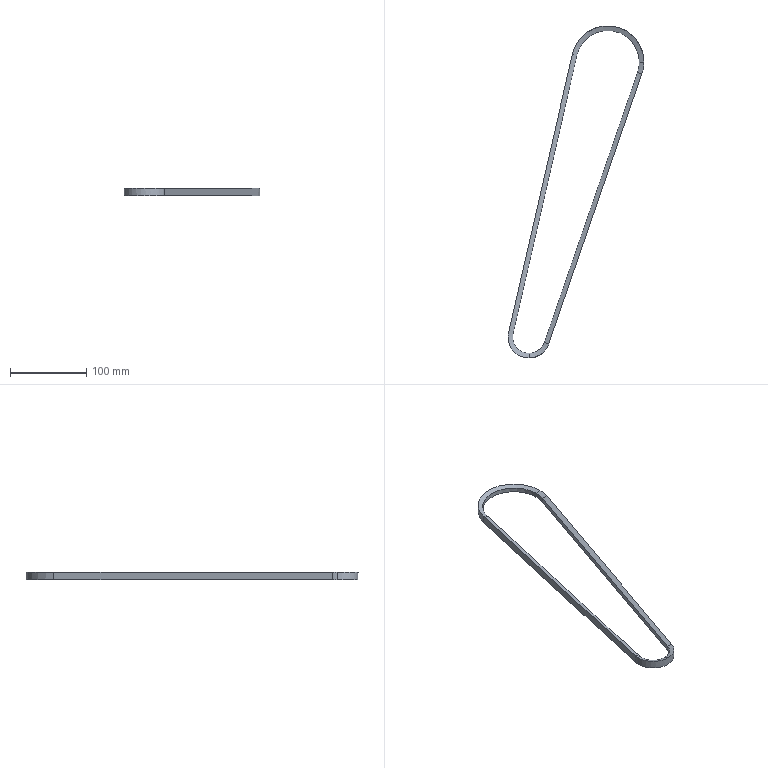Part | SolidWorks | features BaseBody 1 | 1 solid | 21 faces | box 178.368 x 436.001 x 10.319 mm | volume 47372 mm3 | plane 8 | cone 7 | cylinder 6 | commonest cylinder face diameters 42.997 x2 54.997 x2 82.997 x1 94.997 x1
STEP:
#1=CARTESIAN_POINT('',(-103.371,-375.002,5.159));
#2=VERTEX_POINT('',#1);
#3=CARTESIAN_POINT('',(-130.869,-347.503,5.159));
#4=VERTEX_POINT('',#3);
#5=CARTESIAN_POINT('',(-103.371,-347.503,5.159));
#6=DIRECTION('',(0.,0.,-1.));
#7=DIRECTION('',(-1.,0.,0.));
#8=AXIS2_PLACEMENT_3D('',#5,#6,#7);
#9=CIRCLE('',#8,27.499);
#10=EDGE_CURVE('',#2,#4,#9,.T.);
#11=ORIENTED_EDGE('',*,*,#10,.T.);
#12=CARTESIAN_POINT('',(-130.869,-347.503,-5.159));
#13=VERTEX_POINT('',#12);
#14=CARTESIAN_POINT('',(-130.869,-347.503,0.));
#15=DIRECTION('',(0.,0.,-1.));
#16=VECTOR('',#15,1000.);
#17=LINE('',#14,#16);
#18=EDGE_CURVE('',#4,#13,#17,.T.);
#19=ORIENTED_EDGE('',*,*,#18,.T.);
#20=CARTESIAN_POINT('',(-77.375,-356.47,-5.159));
#21=VERTEX_POINT('',#20);
#22=CARTESIAN_POINT('',(-103.371,-347.503,-5.159));
#23=DIRECTION('',(0.,0.,1.));
#24=DIRECTION('',(-1.,0.,0.));
#25=AXIS2_PLACEMENT_3D('',#22,#23,#24);
#26=CIRCLE('',#25,27.499);
#27=EDGE_CURVE('',#13,#21,#26,.T.);
#28=ORIENTED_EDGE('',*,*,#27,.T.);
#29=CARTESIAN_POINT('',(-77.375,-356.47,5.159));
#30=VERTEX_POINT('',#29);
#31=CARTESIAN_POINT('',(-77.375,-356.47,5.159));
#32=DIRECTION('',(0.,0.,-1.));
#33=VECTOR('',#32,1000.);
#34=LINE('',#31,#33);
#35=EDGE_CURVE('',#30,#21,#34,.T.);
#36=ORIENTED_EDGE('',*,*,#35,.F.);
#37=CARTESIAN_POINT('',(-103.371,-347.503,5.159));
#38=DIRECTION('',(0.,0.,-1.));
#39=DIRECTION('',(-1.,0.,0.));
#40=AXIS2_PLACEMENT_3D('',#37,#38,#39);
#41=CIRCLE('',#40,27.499);
#42=EDGE_CURVE('',#30,#2,#41,.T.);
#43=ORIENTED_EDGE('',*,*,#42,.T.);
#44=EDGE_LOOP('',(#11,#19,#28,#36,#43));
#45=FACE_OUTER_BOUND('',#44,.T.);
#46=CARTESIAN_POINT('',(-103.371,-347.503,0.));
#47=DIRECTION('',(0.,0.,-1.));
#48=DIRECTION('',(-1.,0.,0.));
#49=AXIS2_PLACEMENT_3D('',#46,#47,#48);
#50=CYLINDRICAL_SURFACE('',#49,27.499);
#51=ADVANCED_FACE('',(#45),#50,.T.);
#52=CARTESIAN_POINT('',(41.499,13.5,2.976));
#53=VERTEX_POINT('',#52);
#54=CARTESIAN_POINT('',(-40.447,22.783,2.976));
#55=VERTEX_POINT('',#54);
#56=CARTESIAN_POINT('',(0.,13.5,2.976));
#57=DIRECTION('',(0.,0.,1.));
#58=DIRECTION('',(-0.9453,0.3261,0.));
#59=AXIS2_PLACEMENT_3D('',#56,#57,#58);
#60=CIRCLE('',#59,41.499);
#61=EDGE_CURVE('',#53,#55,#60,.T.);
#62=ORIENTED_EDGE('',*,*,#61,.F.);
#63=CARTESIAN_POINT('',(47.499,13.5,5.159));
#64=VERTEX_POINT('',#63);
#65=CARTESIAN_POINT('',(47.499,13.5,5.159));
#66=DIRECTION('',(0.9397,0.,0.342));
#67=VECTOR('',#66,1000.);
#68=LINE('',#65,#67);
#69=EDGE_CURVE('',#53,#64,#68,.T.);
#70=ORIENTED_EDGE('',*,*,#69,.T.);
#71=CARTESIAN_POINT('',(-46.295,24.125,5.159));
#72=VERTEX_POINT('',#71);
#73=CARTESIAN_POINT('',(0.,13.5,5.159));
#74=DIRECTION('',(0.,0.,-1.));
#75=DIRECTION('',(-1.,0.,0.));
#76=AXIS2_PLACEMENT_3D('',#73,#74,#75);
#77=CIRCLE('',#76,47.499);
#78=EDGE_CURVE('',#72,#64,#77,.T.);
#79=ORIENTED_EDGE('',*,*,#78,.F.);
#80=CARTESIAN_POINT('',(-43.371,23.454,4.068));
#81=DIRECTION('',(-0.9159,0.2102,0.342));
#82=VECTOR('',#81,1000.);
#83=LINE('',#80,#82);
#84=EDGE_CURVE('',#55,#72,#83,.T.);
#85=ORIENTED_EDGE('',*,*,#84,.F.);
#86=EDGE_LOOP('',(#62,#70,#79,#85));
#87=FACE_OUTER_BOUND('',#86,.T.);
#88=CARTESIAN_POINT('',(0.,13.5,5.159));
#89=DIRECTION('',(0.,0.,1.));
#90=DIRECTION('',(1.,0.,0.));
#91=AXIS2_PLACEMENT_3D('',#88,#89,#90);
#92=CONICAL_SURFACE('',#91,47.499,1.222);
#93=ADVANCED_FACE('',(#87),#92,.F.);
#94=CARTESIAN_POINT('',(-103.371,-369.002,2.976));
#95=VERTEX_POINT('',#94);
#96=CARTESIAN_POINT('',(-83.047,-354.514,2.976));
#97=VERTEX_POINT('',#96);
#98=CARTESIAN_POINT('',(-103.371,-347.503,2.976));
#99=DIRECTION('',(0.,0.,1.));
#100=DIRECTION('',(0.9747,-0.2237,0.));
#101=AXIS2_PLACEMENT_3D('',#98,#99,#100);
#102=CIRCLE('',#101,21.499);
#103=EDGE_CURVE('',#95,#97,#102,.T.);
#104=ORIENTED_EDGE('',*,*,#103,.F.);
#105=CARTESIAN_POINT('',(-103.371,-375.002,5.159));
#106=DIRECTION('',(0.,-0.9397,0.342));
#107=VECTOR('',#106,1000.);
#108=LINE('',#105,#107);
#109=EDGE_CURVE('',#95,#2,#108,.T.);
#110=ORIENTED_EDGE('',*,*,#109,.T.);
#111=ORIENTED_EDGE('',*,*,#42,.F.);
#112=CARTESIAN_POINT('',(-83.047,-354.514,2.976));
#113=DIRECTION('',(0.8883,-0.3064,0.342));
#114=VECTOR('',#113,1000.);
#115=LINE('',#112,#114);
#116=EDGE_CURVE('',#97,#30,#115,.T.);
#117=ORIENTED_EDGE('',*,*,#116,.F.);
#118=EDGE_LOOP('',(#104,#110,#111,#117));
#119=FACE_OUTER_BOUND('',#118,.T.);
#120=CARTESIAN_POINT('',(-103.371,-347.503,5.159));
#121=DIRECTION('',(0.,0.,1.));
#122=DIRECTION('',(0.,-1.,0.));
#123=AXIS2_PLACEMENT_3D('',#120,#121,#122);
#124=CONICAL_SURFACE('',#123,27.499,1.222);
#125=ADVANCED_FACE('',(#119),#124,.F.);
#126=CARTESIAN_POINT('',(-124.869,-347.503,-2.976));
#127=VERTEX_POINT('',#126);
#128=CARTESIAN_POINT('',(-124.325,-342.694,-2.976));
#129=VERTEX_POINT('',#128);
#130=CARTESIAN_POINT('',(-103.371,-347.503,-2.976));
#131=DIRECTION('',(0.,0.,-1.));
#132=DIRECTION('',(0.9747,-0.2237,0.));
#133=AXIS2_PLACEMENT_3D('',#130,#131,#132);
#134=CIRCLE('',#133,21.499);
#135=EDGE_CURVE('',#127,#129,#134,.T.);
#136=ORIENTED_EDGE('',*,*,#135,.F.);
#137=CARTESIAN_POINT('',(-130.869,-347.503,-5.159));
#138=DIRECTION('',(-0.9397,0.,-0.342));
#139=VECTOR('',#138,1000.);
#140=LINE('',#137,#139);
#141=EDGE_CURVE('',#127,#13,#140,.T.);
#142=ORIENTED_EDGE('',*,*,#141,.T.);
#143=CARTESIAN_POINT('',(-130.173,-341.352,-5.159));
#144=VERTEX_POINT('',#143);
#145=CARTESIAN_POINT('',(-103.371,-347.503,-5.159));
#146=DIRECTION('',(0.,0.,1.));
#147=DIRECTION('',(-1.,0.,0.));
#148=AXIS2_PLACEMENT_3D('',#145,#146,#147);
#149=CIRCLE('',#148,27.499);
#150=EDGE_CURVE('',#144,#13,#149,.T.);
#151=ORIENTED_EDGE('',*,*,#150,.F.);
#152=CARTESIAN_POINT('',(-127.249,-342.023,-4.068));
#153=DIRECTION('',(-0.9159,0.2102,-0.342));
#154=VECTOR('',#153,1000.);
#155=LINE('',#152,#154);
#156=EDGE_CURVE('',#129,#144,#155,.T.);
#157=ORIENTED_EDGE('',*,*,#156,.F.);
#158=EDGE_LOOP('',(#136,#142,#151,#157));
#159=FACE_OUTER_BOUND('',#158,.T.);
#160=CARTESIAN_POINT('',(-103.371,-347.503,-5.159));
#161=DIRECTION('',(0.,0.,-1.));
#162=DIRECTION('',(-1.,0.,0.));
#163=AXIS2_PLACEMENT_3D('',#160,#161,#162);
#164=CONICAL_SURFACE('',#163,27.499,1.222);
#165=ADVANCED_FACE('',(#159),#164,.F.);
#166=CARTESIAN_POINT('',(-124.325,-342.694,2.976));
#167=VERTEX_POINT('',#166);
#168=CARTESIAN_POINT('',(-124.869,-347.503,2.976));
#169=VERTEX_POINT('',#168);
#170=CARTESIAN_POINT('',(-103.371,-347.503,2.976));
#171=DIRECTION('',(0.,0.,1.));
#172=DIRECTION('',(0.9747,-0.2237,0.));
#173=AXIS2_PLACEMENT_3D('',#170,#171,#172);
#174=CIRCLE('',#173,21.499);
#175=EDGE_CURVE('',#167,#169,#174,.T.);
#176=ORIENTED_EDGE('',*,*,#175,.T.);
#177=CARTESIAN_POINT('',(-124.869,-347.503,0.));
#178=DIRECTION('',(0.,0.,-1.));
#179=VECTOR('',#178,1000.);
#180=LINE('',#177,#179);
#181=EDGE_CURVE('',#169,#127,#180,.T.);
#182=ORIENTED_EDGE('',*,*,#181,.T.);
#183=ORIENTED_EDGE('',*,*,#135,.T.);
#184=CARTESIAN_POINT('',(-124.325,-342.694,0.));
#185=DIRECTION('',(0.,0.,-1.));
#186=VECTOR('',#185,1000.);
#187=LINE('',#184,#186);
#188=EDGE_CURVE('',#167,#129,#187,.T.);
#189=ORIENTED_EDGE('',*,*,#188,.F.);
#190=EDGE_LOOP('',(#176,#182,#183,#189));
#191=FACE_OUTER_BOUND('',#190,.T.);
#192=CARTESIAN_POINT('',(-103.371,-347.503,0.));
#193=DIRECTION('',(0.,0.,-1.));
#194=DIRECTION('',(-1.,0.,0.));
#195=AXIS2_PLACEMENT_3D('',#192,#193,#194);
#196=CYLINDRICAL_SURFACE('',#195,21.499);
#197=ADVANCED_FACE('',(#191),#196,.F.);
#198=CARTESIAN_POINT('',(44.902,-1.989,-5.159));
#199=VERTEX_POINT('',#198);
#200=CARTESIAN_POINT('',(44.902,-1.989,5.159));
#201=VERTEX_POINT('',#200);
#202=CARTESIAN_POINT('',(44.902,-1.989,5.159));
#203=DIRECTION('',(0.,0.,1.));
#204=VECTOR('',#203,1000.);
#205=LINE('',#202,#204);
#206=EDGE_CURVE('',#199,#201,#205,.T.);
#207=ORIENTED_EDGE('',*,*,#206,.T.);
#208=CARTESIAN_POINT('',(44.902,-1.989,5.159));
#209=DIRECTION('',(-0.3261,-0.9453,0.));
#210=VECTOR('',#209,1000.);
#211=LINE('',#208,#210);
#212=EDGE_CURVE('',#201,#30,#211,.T.);
#213=ORIENTED_EDGE('',*,*,#212,.T.);
#214=ORIENTED_EDGE('',*,*,#35,.T.);
#215=CARTESIAN_POINT('',(44.902,-1.989,-5.159));
#216=DIRECTION('',(0.3261,0.9453,0.));
#217=VECTOR('',#216,1000.);
#218=LINE('',#215,#217);
#219=EDGE_CURVE('',#21,#199,#218,.T.);
#220=ORIENTED_EDGE('',*,*,#219,.T.);
#221=EDGE_LOOP('',(#207,#213,#214,#220));
#222=FACE_OUTER_BOUND('',#221,.T.);
#223=CARTESIAN_POINT('',(44.902,-1.989,5.159));
#224=DIRECTION('',(0.9453,-0.3261,0.));
#225=DIRECTION('',(0.3261,0.9453,0.));
#226=AXIS2_PLACEMENT_3D('',#223,#224,#225);
#227=PLANE('',#226);
#228=ADVANCED_FACE('',(#222),#227,.T.);
#229=CARTESIAN_POINT('',(39.23,-0.03236,2.976));
#230=VERTEX_POINT('',#229);
#231=CARTESIAN_POINT('',(44.902,-1.989,5.159));
#232=DIRECTION('',(-0.8883,0.3064,-0.342));
#233=VECTOR('',#232,1000.);
#234=LINE('',#231,#233);
#235=EDGE_CURVE('',#201,#230,#234,.T.);
#236=ORIENTED_EDGE('',*,*,#235,.T.);
#237=CARTESIAN_POINT('',(39.23,-0.03236,2.976));
#238=DIRECTION('',(-0.3261,-0.9453,0.));
#239=VECTOR('',#238,1000.);
#240=LINE('',#237,#239);
#241=EDGE_CURVE('',#230,#97,#240,.T.);
#242=ORIENTED_EDGE('',*,*,#241,.T.);
#243=ORIENTED_EDGE('',*,*,#116,.T.);
#244=ORIENTED_EDGE('',*,*,#212,.F.);
#245=EDGE_LOOP('',(#236,#242,#243,#244));
#246=FACE_OUTER_BOUND('',#245,.T.);
#247=CARTESIAN_POINT('',(39.23,-0.03236,2.976));
#248=DIRECTION('',(-0.3233,0.1115,0.9397));
#249=DIRECTION('',(0.9456,0.,0.3254));
#250=AXIS2_PLACEMENT_3D('',#247,#248,#249);
#251=PLANE('',#250);
#252=ADVANCED_FACE('',(#246),#251,.T.);
#253=CARTESIAN_POINT('',(-46.295,24.125,-5.159));
#254=VERTEX_POINT('',#253);
#255=CARTESIAN_POINT('',(-46.295,24.125,0.));
#256=DIRECTION('',(0.,0.,1.));
#257=VECTOR('',#256,1000.);
#258=LINE('',#255,#257);
#259=EDGE_CURVE('',#254,#72,#258,.T.);
#260=ORIENTED_EDGE('',*,*,#259,.T.);
#261=ORIENTED_EDGE('',*,*,#78,.T.);
#262=CARTESIAN_POINT('',(0.,13.5,5.159));
#263=DIRECTION('',(0.,0.,-1.));
#264=DIRECTION('',(-1.,0.,0.));
#265=AXIS2_PLACEMENT_3D('',#262,#263,#264);
#266=CIRCLE('',#265,47.499);
#267=EDGE_CURVE('',#64,#201,#266,.T.);
#268=ORIENTED_EDGE('',*,*,#267,.T.);
#269=ORIENTED_EDGE('',*,*,#206,.F.);
#270=CARTESIAN_POINT('',(0.,13.5,-5.159));
#271=DIRECTION('',(0.,0.,1.));
#272=DIRECTION('',(-1.,0.,0.));
#273=AXIS2_PLACEMENT_3D('',#270,#271,#272);
#274=CIRCLE('',#273,47.499);
#275=EDGE_CURVE('',#199,#254,#274,.T.);
#276=ORIENTED_EDGE('',*,*,#275,.T.);
#277=EDGE_LOOP('',(#260,#261,#268,#269,#276));
#278=FACE_OUTER_BOUND('',#277,.T.);
#279=CARTESIAN_POINT('',(0.,13.5,0.));
#280=DIRECTION('',(0.,0.,-1.));
#281=DIRECTION('',(-1.,0.,0.));
#282=AXIS2_PLACEMENT_3D('',#279,#280,#281);
#283=CYLINDRICAL_SURFACE('',#282,47.499);
#284=ADVANCED_FACE('',(#278),#283,.T.);
#285=CARTESIAN_POINT('',(39.23,-0.03236,-2.976));
#286=VERTEX_POINT('',#285);
#287=CARTESIAN_POINT('',(39.23,-0.03236,-2.976));
#288=DIRECTION('',(0.8883,-0.3064,-0.342));
#289=VECTOR('',#288,1000.);
#290=LINE('',#287,#289);
#291=EDGE_CURVE('',#286,#199,#290,.T.);
#292=ORIENTED_EDGE('',*,*,#291,.T.);
#293=ORIENTED_EDGE('',*,*,#219,.F.);
#294=CARTESIAN_POINT('',(-83.047,-354.514,-2.976));
#295=VERTEX_POINT('',#294);
#296=CARTESIAN_POINT('',(-77.375,-356.47,-5.159));
#297=DIRECTION('',(-0.8883,0.3064,0.342));
#298=VECTOR('',#297,1000.);
#299=LINE('',#296,#298);
#300=EDGE_CURVE('',#21,#295,#299,.T.);
#301=ORIENTED_EDGE('',*,*,#300,.T.);
#302=CARTESIAN_POINT('',(-83.047,-354.514,-2.976));
#303=DIRECTION('',(0.3261,0.9453,0.));
#304=VECTOR('',#303,1000.);
#305=LINE('',#302,#304);
#306=EDGE_CURVE('',#295,#286,#305,.T.);
#307=ORIENTED_EDGE('',*,*,#306,.T.);
#308=EDGE_LOOP('',(#292,#293,#301,#307));
#309=FACE_OUTER_BOUND('',#308,.T.);
#310=CARTESIAN_POINT('',(44.902,-1.989,-5.159));
#311=DIRECTION('',(-0.3233,0.1115,-0.9397));
#312=DIRECTION('',(-0.9456,0.,0.3254));
#313=AXIS2_PLACEMENT_3D('',#310,#311,#312);
#314=PLANE('',#313);
#315=ADVANCED_FACE('',(#309),#314,.T.);
#316=ORIENTED_EDGE('',*,*,#18,.F.);
#317=CARTESIAN_POINT('',(-130.173,-341.352,5.159));
#318=VERTEX_POINT('',#317);
#319=CARTESIAN_POINT('',(-103.371,-347.503,5.159));
#320=DIRECTION('',(0.,0.,-1.));
#321=DIRECTION('',(-1.,0.,0.));
#322=AXIS2_PLACEMENT_3D('',#319,#320,#321);
#323=CIRCLE('',#322,27.499);
#324=EDGE_CURVE('',#4,#318,#323,.T.);
#325=ORIENTED_EDGE('',*,*,#324,.T.);
#326=CARTESIAN_POINT('',(-130.173,-341.352,0.));
#327=DIRECTION('',(0.,0.,-1.));
#328=VECTOR('',#327,1000.);
#329=LINE('',#326,#328);
#330=EDGE_CURVE('',#318,#144,#329,.T.);
#331=ORIENTED_EDGE('',*,*,#330,.T.);
#332=ORIENTED_EDGE('',*,*,#150,.T.);
#333=EDGE_LOOP('',(#316,#325,#331,#332));
#334=FACE_OUTER_BOUND('',#333,.T.);
#335=CARTESIAN_POINT('',(-103.371,-347.503,0.));
#336=DIRECTION('',(0.,0.,-1.));
#337=DIRECTION('',(-1.,0.,0.));
#338=AXIS2_PLACEMENT_3D('',#335,#336,#337);
#339=CYLINDRICAL_SURFACE('',#338,27.499);
#340=ADVANCED_FACE('',(#334),#339,.T.);
#341=CARTESIAN_POINT('',(39.23,-0.03236,-2.976));
#342=DIRECTION('',(0.,0.,-1.));
#343=VECTOR('',#342,1000.);
#344=LINE('',#341,#343);
#345=EDGE_CURVE('',#230,#286,#344,.T.);
#346=ORIENTED_EDGE('',*,*,#345,.T.);
#347=ORIENTED_EDGE('',*,*,#306,.F.);
#348=CARTESIAN_POINT('',(-83.047,-354.514,-2.976));
#349=DIRECTION('',(0.,0.,1.));
#350=VECTOR('',#349,1000.);
#351=LINE('',#348,#350);
#352=EDGE_CURVE('',#295,#97,#351,.T.);
#353=ORIENTED_EDGE('',*,*,#352,.T.);
#354=ORIENTED_EDGE('',*,*,#241,.F.);
#355=EDGE_LOOP('',(#346,#347,#353,#354));
#356=FACE_OUTER_BOUND('',#355,.T.);
#357=CARTESIAN_POINT('',(39.23,-0.03236,-2.976));
#358=DIRECTION('',(-0.9453,0.3261,0.));
#359=DIRECTION('',(-0.3261,-0.9453,0.));
#360=AXIS2_PLACEMENT_3D('',#357,#358,#359);
#361=PLANE('',#360);
#362=ADVANCED_FACE('',(#356),#361,.T.);
#363=ORIENTED_EDGE('',*,*,#69,.F.);
#364=CARTESIAN_POINT('',(0.,13.5,2.976));
#365=DIRECTION('',(0.,0.,1.));
#366=DIRECTION('',(-0.9453,0.3261,0.));
#367=AXIS2_PLACEMENT_3D('',#364,#365,#366);
#368=CIRCLE('',#367,41.499);
#369=EDGE_CURVE('',#230,#53,#368,.T.);
#370=ORIENTED_EDGE('',*,*,#369,.F.);
#371=ORIENTED_EDGE('',*,*,#235,.F.);
#372=ORIENTED_EDGE('',*,*,#267,.F.);
#373=EDGE_LOOP('',(#363,#370,#371,#372));
#374=FACE_OUTER_BOUND('',#373,.T.);
#375=CARTESIAN_POINT('',(0.,13.5,5.159));
#376=DIRECTION('',(0.,0.,1.));
#377=DIRECTION('',(1.,0.,0.));
#378=AXIS2_PLACEMENT_3D('',#375,#376,#377);
#379=CONICAL_SURFACE('',#378,47.499,1.222);
#380=ADVANCED_FACE('',(#374),#379,.F.);
#381=ORIENTED_EDGE('',*,*,#109,.F.);
#382=CARTESIAN_POINT('',(-103.371,-347.503,2.976));
#383=DIRECTION('',(0.,0.,1.));
#384=DIRECTION('',(0.9747,-0.2237,0.));
#385=AXIS2_PLACEMENT_3D('',#382,#383,#384);
#386=CIRCLE('',#385,21.499);
#387=EDGE_CURVE('',#169,#95,#386,.T.);
#388=ORIENTED_EDGE('',*,*,#387,.F.);
#389=ORIENTED_EDGE('',*,*,#175,.F.);
#390=CARTESIAN_POINT('',(-127.249,-342.023,4.068));
#391=DIRECTION('',(0.9159,-0.2102,-0.342));
#392=VECTOR('',#391,1000.);
#393=LINE('',#390,#392);
#394=EDGE_CURVE('',#318,#167,#393,.T.);
#395=ORIENTED_EDGE('',*,*,#394,.F.);
#396=ORIENTED_EDGE('',*,*,#324,.F.);
#397=ORIENTED_EDGE('',*,*,#10,.F.);
#398=EDGE_LOOP('',(#381,#388,#389,#395,#396,#397));
#399=FACE_OUTER_BOUND('',#398,.T.);
#400=CARTESIAN_POINT('',(-103.371,-347.503,5.159));
#401=DIRECTION('',(0.,0.,1.));
#402=DIRECTION('',(0.,-1.,0.));
#403=AXIS2_PLACEMENT_3D('',#400,#401,#402);
#404=CONICAL_SURFACE('',#403,27.499,1.222);
#405=ADVANCED_FACE('',(#399),#404,.F.);
#406=ORIENTED_EDGE('',*,*,#330,.F.);
#407=CARTESIAN_POINT('',(-130.173,-341.352,5.159));
#408=DIRECTION('',(0.2237,0.9747,0.));
#409=VECTOR('',#408,1000.);
#410=LINE('',#407,#409);
#411=EDGE_CURVE('',#318,#72,#410,.T.);
#412=ORIENTED_EDGE('',*,*,#411,.T.);
#413=ORIENTED_EDGE('',*,*,#259,.F.);
#414=CARTESIAN_POINT('',(-130.173,-341.352,-5.159));
#415=DIRECTION('',(-0.2237,-0.9747,0.));
#416=VECTOR('',#415,1000.);
#417=LINE('',#414,#416);
#418=EDGE_CURVE('',#254,#144,#417,.T.);
#419=ORIENTED_EDGE('',*,*,#418,.T.);
#420=EDGE_LOOP('',(#406,#412,#413,#419));
#421=FACE_OUTER_BOUND('',#420,.T.);
#422=CARTESIAN_POINT('',(-130.173,-341.352,5.159));
#423=DIRECTION('',(-0.9747,0.2237,0.));
#424=DIRECTION('',(-0.2237,-0.9747,0.));
#425=AXIS2_PLACEMENT_3D('',#422,#423,#424);
#426=PLANE('',#425);
#427=ADVANCED_FACE('',(#421),#426,.T.);
#428=CARTESIAN_POINT('',(-40.447,22.783,-2.976));
#429=VERTEX_POINT('',#428);
#430=CARTESIAN_POINT('',(0.,13.5,-2.976));
#431=DIRECTION('',(0.,0.,-1.));
#432=DIRECTION('',(-0.9453,0.3261,0.));
#433=AXIS2_PLACEMENT_3D('',#430,#431,#432);
#434=CIRCLE('',#433,41.499);
#435=EDGE_CURVE('',#429,#286,#434,.T.);
#436=ORIENTED_EDGE('',*,*,#435,.F.);
#437=CARTESIAN_POINT('',(-43.371,23.454,-4.068));
#438=DIRECTION('',(0.9159,-0.2102,0.342));
#439=VECTOR('',#438,1000.);
#440=LINE('',#437,#439);
#441=EDGE_CURVE('',#254,#429,#440,.T.);
#442=ORIENTED_EDGE('',*,*,#441,.F.);
#443=ORIENTED_EDGE('',*,*,#275,.F.);
#444=ORIENTED_EDGE('',*,*,#291,.F.);
#445=EDGE_LOOP('',(#436,#442,#443,#444));
#446=FACE_OUTER_BOUND('',#445,.T.);
#447=CARTESIAN_POINT('',(0.,13.5,-5.159));
#448=DIRECTION('',(0.,0.,-1.));
#449=DIRECTION('',(-1.,0.,0.));
#450=AXIS2_PLACEMENT_3D('',#447,#448,#449);
#451=CONICAL_SURFACE('',#450,47.499,1.222);
#452=ADVANCED_FACE('',(#446),#451,.F.);
#453=ORIENTED_EDGE('',*,*,#141,.F.);
#454=CARTESIAN_POINT('',(-103.371,-347.503,-2.976));
#455=DIRECTION('',(0.,0.,-1.));
#456=DIRECTION('',(0.9747,-0.2237,0.));
#457=AXIS2_PLACEMENT_3D('',#454,#455,#456);
#458=CIRCLE('',#457,21.499);
#459=EDGE_CURVE('',#295,#127,#458,.T.);
#460=ORIENTED_EDGE('',*,*,#459,.F.);
#461=ORIENTED_EDGE('',*,*,#300,.F.);
#462=ORIENTED_EDGE('',*,*,#27,.F.);
#463=EDGE_LOOP('',(#453,#460,#461,#462));
#464=FACE_OUTER_BOUND('',#463,.T.);
#465=CARTESIAN_POINT('',(-103.371,-347.503,-5.159));
#466=DIRECTION('',(0.,0.,-1.));
#467=DIRECTION('',(-1.,0.,0.));
#468=AXIS2_PLACEMENT_3D('',#465,#466,#467);
#469=CONICAL_SURFACE('',#468,27.499,1.222);
#470=ADVANCED_FACE('',(#464),#469,.F.);
#471=ORIENTED_EDGE('',*,*,#369,.T.);
#472=ORIENTED_EDGE('',*,*,#61,.T.);
#473=CARTESIAN_POINT('',(-40.447,22.783,0.));
#474=DIRECTION('',(0.,0.,1.));
#475=VECTOR('',#474,1000.);
#476=LINE('',#473,#475);
#477=EDGE_CURVE('',#429,#55,#476,.T.);
#478=ORIENTED_EDGE('',*,*,#477,.F.);
#479=ORIENTED_EDGE('',*,*,#435,.T.);
#480=ORIENTED_EDGE('',*,*,#345,.F.);
#481=EDGE_LOOP('',(#471,#472,#478,#479,#480));
#482=FACE_OUTER_BOUND('',#481,.T.);
#483=CARTESIAN_POINT('',(0.,13.5,0.));
#484=DIRECTION('',(0.,0.,-1.));
#485=DIRECTION('',(-1.,0.,0.));
#486=AXIS2_PLACEMENT_3D('',#483,#484,#485);
#487=CYLINDRICAL_SURFACE('',#486,41.499);
#488=ADVANCED_FACE('',(#482),#487,.F.);
#489=ORIENTED_EDGE('',*,*,#181,.F.);
#490=ORIENTED_EDGE('',*,*,#387,.T.);
#491=ORIENTED_EDGE('',*,*,#103,.T.);
#492=ORIENTED_EDGE('',*,*,#352,.F.);
#493=ORIENTED_EDGE('',*,*,#459,.T.);
#494=EDGE_LOOP('',(#489,#490,#491,#492,#493));
#495=FACE_OUTER_BOUND('',#494,.T.);
#496=CARTESIAN_POINT('',(-103.371,-347.503,0.));
#497=DIRECTION('',(0.,0.,-1.));
#498=DIRECTION('',(-1.,0.,0.));
#499=AXIS2_PLACEMENT_3D('',#496,#497,#498);
#500=CYLINDRICAL_SURFACE('',#499,21.499);
#501=ADVANCED_FACE('',(#495),#500,.F.);
#502=ORIENTED_EDGE('',*,*,#394,.T.);
#503=CARTESIAN_POINT('',(-124.325,-342.694,2.976));
#504=DIRECTION('',(0.2237,0.9747,0.));
#505=VECTOR('',#504,1000.);
#506=LINE('',#503,#505);
#507=EDGE_CURVE('',#167,#55,#506,.T.);
#508=ORIENTED_EDGE('',*,*,#507,.T.);
#509=ORIENTED_EDGE('',*,*,#84,.T.);
#510=ORIENTED_EDGE('',*,*,#411,.F.);
#511=EDGE_LOOP('',(#502,#508,#509,#510));
#512=FACE_OUTER_BOUND('',#511,.T.);
#513=CARTESIAN_POINT('',(-124.325,-342.694,2.976));
#514=DIRECTION('',(0.3334,-0.07651,0.9397));
#515=DIRECTION('',(0.9425,0.,-0.3343));
#516=AXIS2_PLACEMENT_3D('',#513,#514,#515);
#517=PLANE('',#516);
#518=ADVANCED_FACE('',(#512),#517,.T.);
#519=ORIENTED_EDGE('',*,*,#156,.T.);
#520=ORIENTED_EDGE('',*,*,#418,.F.);
#521=ORIENTED_EDGE('',*,*,#441,.T.);
#522=CARTESIAN_POINT('',(-40.447,22.783,-2.976));
#523=DIRECTION('',(-0.2237,-0.9747,0.));
#524=VECTOR('',#523,1000.);
#525=LINE('',#522,#524);
#526=EDGE_CURVE('',#429,#129,#525,.T.);
#527=ORIENTED_EDGE('',*,*,#526,.T.);
#528=EDGE_LOOP('',(#519,#520,#521,#527));
#529=FACE_OUTER_BOUND('',#528,.T.);
#530=CARTESIAN_POINT('',(-130.173,-341.352,-5.159));
#531=DIRECTION('',(0.3334,-0.07651,-0.9397));
#532=DIRECTION('',(-0.9425,0.,-0.3343));
#533=AXIS2_PLACEMENT_3D('',#530,#531,#532);
#534=PLANE('',#533);
#535=ADVANCED_FACE('',(#529),#534,.T.);
#536=ORIENTED_EDGE('',*,*,#188,.T.);
#537=ORIENTED_EDGE('',*,*,#526,.F.);
#538=ORIENTED_EDGE('',*,*,#477,.T.);
#539=ORIENTED_EDGE('',*,*,#507,.F.);
#540=EDGE_LOOP('',(#536,#537,#538,#539));
#541=FACE_OUTER_BOUND('',#540,.T.);
#542=CARTESIAN_POINT('',(-124.325,-342.694,-2.976));
#543=DIRECTION('',(0.9747,-0.2237,0.));
#544=DIRECTION('',(0.2237,0.9747,0.));
#545=AXIS2_PLACEMENT_3D('',#542,#543,#544);
#546=PLANE('',#545);
#547=ADVANCED_FACE('',(#541),#546,.T.);
#548=CLOSED_SHELL('',(#51,#93,#125,#165,#197,#228,#252,#284,#315,#340,#362,#380,#405,#427,#452,#470,#488,#501,#518,#535,#547));
#549=MANIFOLD_SOLID_BREP('',#548);
#550=CARTESIAN_POINT('',(0.,0.,0.));
#551=DIRECTION('',(0.,0.,1.));
#552=DIRECTION('',(1.,0.,0.));
#553=AXIS2_PLACEMENT_3D('',#550,#551,#552);
#554=(LENGTH_UNIT()NAMED_UNIT(*)SI_UNIT(.MILLI.,.METRE.));
#555=UNCERTAINTY_MEASURE_WITH_UNIT(LENGTH_MEASURE(0.00001),#554,'','');
#556=(NAMED_UNIT(*)PLANE_ANGLE_UNIT()SI_UNIT($,.RADIAN.));
#557=(NAMED_UNIT(*)SI_UNIT($,.STERADIAN.)SOLID_ANGLE_UNIT());
#558=(GEOMETRIC_REPRESENTATION_CONTEXT(3)GLOBAL_UNCERTAINTY_ASSIGNED_CONTEXT((#555))GLOBAL_UNIT_ASSIGNED_CONTEXT((#554,#556,#557))REPRESENTATION_CONTEXT('',''));
#559=ADVANCED_BREP_SHAPE_REPRESENTATION('',(#549,#553),#558);